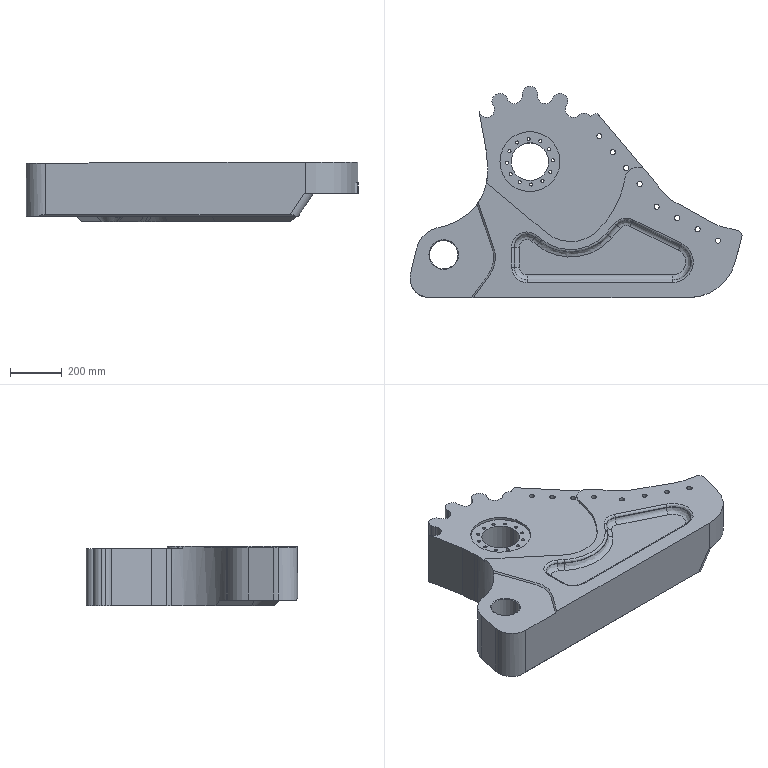Part | SolidWorks | features ICE 7, MoveFace 5, BaseBody 2, Chamfer 1, HoleWzd 1 | 2 solids | 239 faces | box 1278 x 813.2 x 230 mm | volume 107497671 mm3 | cylinder 141 | plane 73 | spline 14 | cone 11 | commonest cylinder face diameters 20 x37 12 x24 60 x13 300 x7 18 x5 40 x5